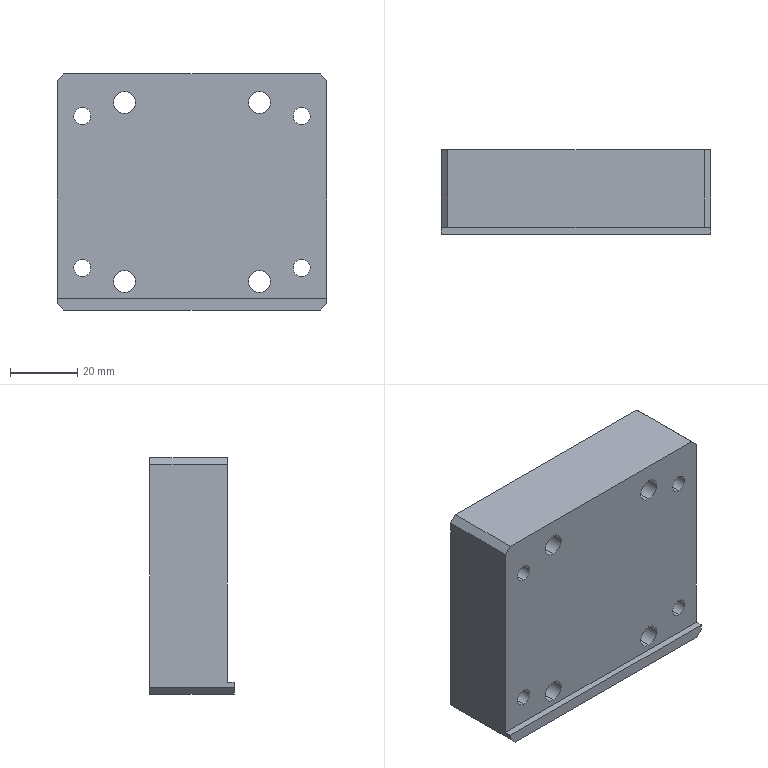Part | SolidWorks | features HoleWzd 3, Chamfer 1, Cut 1, Extrusion 1 | 1 solid | 40 faces | box 80 x 25 x 70 mm | volume 122511 mm3 | cylinder 24 | plane 16 | commonest cylinder face diameters 5 x8 6.6 x8 11 x8
STEP:
#1=CARTESIAN_POINT('',(20.,5.5,-32.));
#2=VERTEX_POINT('',#1);
#3=CARTESIAN_POINT('',(20.,5.5,-21.));
#4=VERTEX_POINT('',#3);
#5=CARTESIAN_POINT('',(20.,5.5,-26.5));
#6=DIRECTION('',(0.,1.,0.));
#7=DIRECTION('',(0.,0.,1.));
#8=AXIS2_PLACEMENT_3D('',#5,#6,#7);
#9=CIRCLE('',#8,5.5);
#10=EDGE_CURVE('',#2,#4,#9,.T.);
#11=ORIENTED_EDGE('',*,*,#10,.F.);
#12=CARTESIAN_POINT('',(20.,12.5,-32.));
#13=VERTEX_POINT('',#12);
#14=CARTESIAN_POINT('',(20.,12.5,-32.));
#15=DIRECTION('',(0.,1.,0.));
#16=VECTOR('',#15,1000.);
#17=LINE('',#14,#16);
#18=EDGE_CURVE('',#2,#13,#17,.T.);
#19=ORIENTED_EDGE('',*,*,#18,.T.);
#20=CARTESIAN_POINT('',(20.,12.5,-21.));
#21=VERTEX_POINT('',#20);
#22=CARTESIAN_POINT('',(20.,12.5,-26.5));
#23=DIRECTION('',(0.,1.,0.));
#24=DIRECTION('',(0.,0.,1.));
#25=AXIS2_PLACEMENT_3D('',#22,#23,#24);
#26=CIRCLE('',#25,5.5);
#27=EDGE_CURVE('',#13,#21,#26,.T.);
#28=ORIENTED_EDGE('',*,*,#27,.T.);
#29=CARTESIAN_POINT('',(20.,12.5,-21.));
#30=DIRECTION('',(0.,1.,0.));
#31=VECTOR('',#30,1000.);
#32=LINE('',#29,#31);
#33=EDGE_CURVE('',#4,#21,#32,.T.);
#34=ORIENTED_EDGE('',*,*,#33,.F.);
#35=EDGE_LOOP('',(#11,#19,#28,#34));
#36=FACE_OUTER_BOUND('',#35,.T.);
#37=CARTESIAN_POINT('',(20.,12.5,-26.5));
#38=DIRECTION('',(0.,1.,0.));
#39=DIRECTION('',(0.,0.,1.));
#40=AXIS2_PLACEMENT_3D('',#37,#38,#39);
#41=CYLINDRICAL_SURFACE('',#40,5.5);
#42=ADVANCED_FACE('',(#36),#41,.F.);
#43=CARTESIAN_POINT('',(20.,-10.5,-29.8));
#44=VERTEX_POINT('',#43);
#45=CARTESIAN_POINT('',(20.,-10.5,-23.2));
#46=VERTEX_POINT('',#45);
#47=CARTESIAN_POINT('',(20.,-10.5,-26.5));
#48=DIRECTION('',(0.,1.,0.));
#49=DIRECTION('',(0.,0.,1.));
#50=AXIS2_PLACEMENT_3D('',#47,#48,#49);
#51=CIRCLE('',#50,3.3);
#52=EDGE_CURVE('',#44,#46,#51,.T.);
#53=ORIENTED_EDGE('',*,*,#52,.F.);
#54=CARTESIAN_POINT('',(20.,5.5,-29.8));
#55=VERTEX_POINT('',#54);
#56=CARTESIAN_POINT('',(20.,12.5,-29.8));
#57=DIRECTION('',(0.,1.,0.));
#58=VECTOR('',#57,1000.);
#59=LINE('',#56,#58);
#60=EDGE_CURVE('',#44,#55,#59,.T.);
#61=ORIENTED_EDGE('',*,*,#60,.T.);
#62=CARTESIAN_POINT('',(20.,5.5,-23.2));
#63=VERTEX_POINT('',#62);
#64=CARTESIAN_POINT('',(20.,5.5,-26.5));
#65=DIRECTION('',(0.,1.,0.));
#66=DIRECTION('',(0.,0.,1.));
#67=AXIS2_PLACEMENT_3D('',#64,#65,#66);
#68=CIRCLE('',#67,3.3);
#69=EDGE_CURVE('',#55,#63,#68,.T.);
#70=ORIENTED_EDGE('',*,*,#69,.T.);
#71=CARTESIAN_POINT('',(20.,12.5,-23.2));
#72=DIRECTION('',(0.,1.,0.));
#73=VECTOR('',#72,1000.);
#74=LINE('',#71,#73);
#75=EDGE_CURVE('',#46,#63,#74,.T.);
#76=ORIENTED_EDGE('',*,*,#75,.F.);
#77=EDGE_LOOP('',(#53,#61,#70,#76));
#78=FACE_OUTER_BOUND('',#77,.T.);
#79=CARTESIAN_POINT('',(20.,12.5,-26.5));
#80=DIRECTION('',(0.,1.,0.));
#81=DIRECTION('',(0.,0.,1.));
#82=AXIS2_PLACEMENT_3D('',#79,#80,#81);
#83=CYLINDRICAL_SURFACE('',#82,3.3);
#84=ADVANCED_FACE('',(#78),#83,.F.);
#85=CARTESIAN_POINT('',(20.,5.5,21.));
#86=VERTEX_POINT('',#85);
#87=CARTESIAN_POINT('',(20.,5.5,32.));
#88=VERTEX_POINT('',#87);
#89=CARTESIAN_POINT('',(20.,5.5,26.5));
#90=DIRECTION('',(0.,1.,0.));
#91=DIRECTION('',(0.,0.,1.));
#92=AXIS2_PLACEMENT_3D('',#89,#90,#91);
#93=CIRCLE('',#92,5.5);
#94=EDGE_CURVE('',#86,#88,#93,.T.);
#95=ORIENTED_EDGE('',*,*,#94,.F.);
#96=CARTESIAN_POINT('',(20.,12.5,21.));
#97=VERTEX_POINT('',#96);
#98=CARTESIAN_POINT('',(20.,12.5,21.));
#99=DIRECTION('',(0.,1.,0.));
#100=VECTOR('',#99,1000.);
#101=LINE('',#98,#100);
#102=EDGE_CURVE('',#86,#97,#101,.T.);
#103=ORIENTED_EDGE('',*,*,#102,.T.);
#104=CARTESIAN_POINT('',(20.,12.5,32.));
#105=VERTEX_POINT('',#104);
#106=CARTESIAN_POINT('',(20.,12.5,26.5));
#107=DIRECTION('',(0.,1.,0.));
#108=DIRECTION('',(0.,0.,1.));
#109=AXIS2_PLACEMENT_3D('',#106,#107,#108);
#110=CIRCLE('',#109,5.5);
#111=EDGE_CURVE('',#97,#105,#110,.T.);
#112=ORIENTED_EDGE('',*,*,#111,.T.);
#113=CARTESIAN_POINT('',(20.,12.5,32.));
#114=DIRECTION('',(0.,1.,0.));
#115=VECTOR('',#114,1000.);
#116=LINE('',#113,#115);
#117=EDGE_CURVE('',#88,#105,#116,.T.);
#118=ORIENTED_EDGE('',*,*,#117,.F.);
#119=EDGE_LOOP('',(#95,#103,#112,#118));
#120=FACE_OUTER_BOUND('',#119,.T.);
#121=CARTESIAN_POINT('',(20.,12.5,26.5));
#122=DIRECTION('',(0.,1.,0.));
#123=DIRECTION('',(0.,0.,1.));
#124=AXIS2_PLACEMENT_3D('',#121,#122,#123);
#125=CYLINDRICAL_SURFACE('',#124,5.5);
#126=ADVANCED_FACE('',(#120),#125,.F.);
#127=CARTESIAN_POINT('',(20.,-10.5,23.2));
#128=VERTEX_POINT('',#127);
#129=CARTESIAN_POINT('',(20.,-10.5,29.8));
#130=VERTEX_POINT('',#129);
#131=CARTESIAN_POINT('',(20.,-10.5,26.5));
#132=DIRECTION('',(0.,1.,0.));
#133=DIRECTION('',(0.,0.,1.));
#134=AXIS2_PLACEMENT_3D('',#131,#132,#133);
#135=CIRCLE('',#134,3.3);
#136=EDGE_CURVE('',#128,#130,#135,.T.);
#137=ORIENTED_EDGE('',*,*,#136,.F.);
#138=CARTESIAN_POINT('',(20.,5.5,23.2));
#139=VERTEX_POINT('',#138);
#140=CARTESIAN_POINT('',(20.,12.5,23.2));
#141=DIRECTION('',(0.,1.,0.));
#142=VECTOR('',#141,1000.);
#143=LINE('',#140,#142);
#144=EDGE_CURVE('',#128,#139,#143,.T.);
#145=ORIENTED_EDGE('',*,*,#144,.T.);
#146=CARTESIAN_POINT('',(20.,5.5,29.8));
#147=VERTEX_POINT('',#146);
#148=CARTESIAN_POINT('',(20.,5.5,26.5));
#149=DIRECTION('',(0.,1.,0.));
#150=DIRECTION('',(0.,0.,1.));
#151=AXIS2_PLACEMENT_3D('',#148,#149,#150);
#152=CIRCLE('',#151,3.3);
#153=EDGE_CURVE('',#139,#147,#152,.T.);
#154=ORIENTED_EDGE('',*,*,#153,.T.);
#155=CARTESIAN_POINT('',(20.,12.5,29.8));
#156=DIRECTION('',(0.,1.,0.));
#157=VECTOR('',#156,1000.);
#158=LINE('',#155,#157);
#159=EDGE_CURVE('',#130,#147,#158,.T.);
#160=ORIENTED_EDGE('',*,*,#159,.F.);
#161=EDGE_LOOP('',(#137,#145,#154,#160));
#162=FACE_OUTER_BOUND('',#161,.T.);
#163=CARTESIAN_POINT('',(20.,12.5,26.5));
#164=DIRECTION('',(0.,1.,0.));
#165=DIRECTION('',(0.,0.,1.));
#166=AXIS2_PLACEMENT_3D('',#163,#164,#165);
#167=CYLINDRICAL_SURFACE('',#166,3.3);
#168=ADVANCED_FACE('',(#162),#167,.F.);
#169=CARTESIAN_POINT('',(-20.,5.5,21.));
#170=VERTEX_POINT('',#169);
#171=CARTESIAN_POINT('',(-20.,5.5,32.));
#172=VERTEX_POINT('',#171);
#173=CARTESIAN_POINT('',(-20.,5.5,26.5));
#174=DIRECTION('',(0.,1.,0.));
#175=DIRECTION('',(0.,0.,1.));
#176=AXIS2_PLACEMENT_3D('',#173,#174,#175);
#177=CIRCLE('',#176,5.5);
#178=EDGE_CURVE('',#170,#172,#177,.T.);
#179=ORIENTED_EDGE('',*,*,#178,.F.);
#180=CARTESIAN_POINT('',(-20.,12.5,21.));
#181=VERTEX_POINT('',#180);
#182=CARTESIAN_POINT('',(-20.,12.5,21.));
#183=DIRECTION('',(0.,1.,0.));
#184=VECTOR('',#183,1000.);
#185=LINE('',#182,#184);
#186=EDGE_CURVE('',#170,#181,#185,.T.);
#187=ORIENTED_EDGE('',*,*,#186,.T.);
#188=CARTESIAN_POINT('',(-20.,12.5,32.));
#189=VERTEX_POINT('',#188);
#190=CARTESIAN_POINT('',(-20.,12.5,26.5));
#191=DIRECTION('',(0.,1.,0.));
#192=DIRECTION('',(0.,0.,1.));
#193=AXIS2_PLACEMENT_3D('',#190,#191,#192);
#194=CIRCLE('',#193,5.5);
#195=EDGE_CURVE('',#181,#189,#194,.T.);
#196=ORIENTED_EDGE('',*,*,#195,.T.);
#197=CARTESIAN_POINT('',(-20.,12.5,32.));
#198=DIRECTION('',(0.,1.,0.));
#199=VECTOR('',#198,1000.);
#200=LINE('',#197,#199);
#201=EDGE_CURVE('',#172,#189,#200,.T.);
#202=ORIENTED_EDGE('',*,*,#201,.F.);
#203=EDGE_LOOP('',(#179,#187,#196,#202));
#204=FACE_OUTER_BOUND('',#203,.T.);
#205=CARTESIAN_POINT('',(-20.,12.5,26.5));
#206=DIRECTION('',(0.,1.,0.));
#207=DIRECTION('',(0.,0.,1.));
#208=AXIS2_PLACEMENT_3D('',#205,#206,#207);
#209=CYLINDRICAL_SURFACE('',#208,5.5);
#210=ADVANCED_FACE('',(#204),#209,.F.);
#211=CARTESIAN_POINT('',(-20.,-10.5,23.2));
#212=VERTEX_POINT('',#211);
#213=CARTESIAN_POINT('',(-20.,-10.5,29.8));
#214=VERTEX_POINT('',#213);
#215=CARTESIAN_POINT('',(-20.,-10.5,26.5));
#216=DIRECTION('',(0.,1.,0.));
#217=DIRECTION('',(0.,0.,1.));
#218=AXIS2_PLACEMENT_3D('',#215,#216,#217);
#219=CIRCLE('',#218,3.3);
#220=EDGE_CURVE('',#212,#214,#219,.T.);
#221=ORIENTED_EDGE('',*,*,#220,.F.);
#222=CARTESIAN_POINT('',(-20.,5.5,23.2));
#223=VERTEX_POINT('',#222);
#224=CARTESIAN_POINT('',(-20.,12.5,23.2));
#225=DIRECTION('',(0.,1.,0.));
#226=VECTOR('',#225,1000.);
#227=LINE('',#224,#226);
#228=EDGE_CURVE('',#212,#223,#227,.T.);
#229=ORIENTED_EDGE('',*,*,#228,.T.);
#230=CARTESIAN_POINT('',(-20.,5.5,29.8));
#231=VERTEX_POINT('',#230);
#232=CARTESIAN_POINT('',(-20.,5.5,26.5));
#233=DIRECTION('',(0.,1.,0.));
#234=DIRECTION('',(0.,0.,1.));
#235=AXIS2_PLACEMENT_3D('',#232,#233,#234);
#236=CIRCLE('',#235,3.3);
#237=EDGE_CURVE('',#223,#231,#236,.T.);
#238=ORIENTED_EDGE('',*,*,#237,.T.);
#239=CARTESIAN_POINT('',(-20.,12.5,29.8));
#240=DIRECTION('',(0.,1.,0.));
#241=VECTOR('',#240,1000.);
#242=LINE('',#239,#241);
#243=EDGE_CURVE('',#214,#231,#242,.T.);
#244=ORIENTED_EDGE('',*,*,#243,.F.);
#245=EDGE_LOOP('',(#221,#229,#238,#244));
#246=FACE_OUTER_BOUND('',#245,.T.);
#247=CARTESIAN_POINT('',(-20.,12.5,26.5));
#248=DIRECTION('',(0.,1.,0.));
#249=DIRECTION('',(0.,0.,1.));
#250=AXIS2_PLACEMENT_3D('',#247,#248,#249);
#251=CYLINDRICAL_SURFACE('',#250,3.3);
#252=ADVANCED_FACE('',(#246),#251,.F.);
#253=CARTESIAN_POINT('',(-20.,5.5,-32.));
#254=VERTEX_POINT('',#253);
#255=CARTESIAN_POINT('',(-20.,5.5,-21.));
#256=VERTEX_POINT('',#255);
#257=CARTESIAN_POINT('',(-20.,5.5,-26.5));
#258=DIRECTION('',(0.,1.,0.));
#259=DIRECTION('',(0.,0.,1.));
#260=AXIS2_PLACEMENT_3D('',#257,#258,#259);
#261=CIRCLE('',#260,5.5);
#262=EDGE_CURVE('',#254,#256,#261,.T.);
#263=ORIENTED_EDGE('',*,*,#262,.F.);
#264=CARTESIAN_POINT('',(-20.,12.5,-32.));
#265=VERTEX_POINT('',#264);
#266=CARTESIAN_POINT('',(-20.,12.5,-32.));
#267=DIRECTION('',(0.,1.,0.));
#268=VECTOR('',#267,1000.);
#269=LINE('',#266,#268);
#270=EDGE_CURVE('',#254,#265,#269,.T.);
#271=ORIENTED_EDGE('',*,*,#270,.T.);
#272=CARTESIAN_POINT('',(-20.,12.5,-21.));
#273=VERTEX_POINT('',#272);
#274=CARTESIAN_POINT('',(-20.,12.5,-26.5));
#275=DIRECTION('',(0.,1.,0.));
#276=DIRECTION('',(0.,0.,1.));
#277=AXIS2_PLACEMENT_3D('',#274,#275,#276);
#278=CIRCLE('',#277,5.5);
#279=EDGE_CURVE('',#265,#273,#278,.T.);
#280=ORIENTED_EDGE('',*,*,#279,.T.);
#281=CARTESIAN_POINT('',(-20.,12.5,-21.));
#282=DIRECTION('',(0.,1.,0.));
#283=VECTOR('',#282,1000.);
#284=LINE('',#281,#283);
#285=EDGE_CURVE('',#256,#273,#284,.T.);
#286=ORIENTED_EDGE('',*,*,#285,.F.);
#287=EDGE_LOOP('',(#263,#271,#280,#286));
#288=FACE_OUTER_BOUND('',#287,.T.);
#289=CARTESIAN_POINT('',(-20.,12.5,-26.5));
#290=DIRECTION('',(0.,1.,0.));
#291=DIRECTION('',(0.,0.,1.));
#292=AXIS2_PLACEMENT_3D('',#289,#290,#291);
#293=CYLINDRICAL_SURFACE('',#292,5.5);
#294=ADVANCED_FACE('',(#288),#293,.F.);
#295=CARTESIAN_POINT('',(-20.,-10.5,-29.8));
#296=VERTEX_POINT('',#295);
#297=CARTESIAN_POINT('',(-20.,-10.5,-23.2));
#298=VERTEX_POINT('',#297);
#299=CARTESIAN_POINT('',(-20.,-10.5,-26.5));
#300=DIRECTION('',(0.,1.,0.));
#301=DIRECTION('',(0.,0.,1.));
#302=AXIS2_PLACEMENT_3D('',#299,#300,#301);
#303=CIRCLE('',#302,3.3);
#304=EDGE_CURVE('',#296,#298,#303,.T.);
#305=ORIENTED_EDGE('',*,*,#304,.F.);
#306=CARTESIAN_POINT('',(-20.,5.5,-29.8));
#307=VERTEX_POINT('',#306);
#308=CARTESIAN_POINT('',(-20.,12.5,-29.8));
#309=DIRECTION('',(0.,1.,0.));
#310=VECTOR('',#309,1000.);
#311=LINE('',#308,#310);
#312=EDGE_CURVE('',#296,#307,#311,.T.);
#313=ORIENTED_EDGE('',*,*,#312,.T.);
#314=CARTESIAN_POINT('',(-20.,5.5,-23.2));
#315=VERTEX_POINT('',#314);
#316=CARTESIAN_POINT('',(-20.,5.5,-26.5));
#317=DIRECTION('',(0.,1.,0.));
#318=DIRECTION('',(0.,0.,1.));
#319=AXIS2_PLACEMENT_3D('',#316,#317,#318);
#320=CIRCLE('',#319,3.3);
#321=EDGE_CURVE('',#307,#315,#320,.T.);
#322=ORIENTED_EDGE('',*,*,#321,.T.);
#323=CARTESIAN_POINT('',(-20.,12.5,-23.2));
#324=DIRECTION('',(0.,1.,0.));
#325=VECTOR('',#324,1000.);
#326=LINE('',#323,#325);
#327=EDGE_CURVE('',#298,#315,#326,.T.);
#328=ORIENTED_EDGE('',*,*,#327,.F.);
#329=EDGE_LOOP('',(#305,#313,#322,#328));
#330=FACE_OUTER_BOUND('',#329,.T.);
#331=CARTESIAN_POINT('',(-20.,12.5,-26.5));
#332=DIRECTION('',(0.,1.,0.));
#333=DIRECTION('',(0.,0.,1.));
#334=AXIS2_PLACEMENT_3D('',#331,#332,#333);
#335=CYLINDRICAL_SURFACE('',#334,3.3);
#336=ADVANCED_FACE('',(#330),#335,.F.);
#337=CARTESIAN_POINT('',(-32.5,12.5,-20.));
#338=VERTEX_POINT('',#337);
#339=CARTESIAN_POINT('',(-32.5,12.5,-25.));
#340=VERTEX_POINT('',#339);
#341=CARTESIAN_POINT('',(-32.5,12.5,-22.5));
#342=DIRECTION('',(0.,-1.,0.));
#343=DIRECTION('',(0.,0.,-1.));
#344=AXIS2_PLACEMENT_3D('',#341,#342,#343);
#345=CIRCLE('',#344,2.5);
#346=EDGE_CURVE('',#338,#340,#345,.T.);
#347=ORIENTED_EDGE('',*,*,#346,.F.);
#348=CARTESIAN_POINT('',(-32.5,-10.5,-20.));
#349=VERTEX_POINT('',#348);
#350=CARTESIAN_POINT('',(-32.5,-10.5,-20.));
#351=DIRECTION('',(0.,-1.,0.));
#352=VECTOR('',#351,1000.);
#353=LINE('',#350,#352);
#354=EDGE_CURVE('',#338,#349,#353,.T.);
#355=ORIENTED_EDGE('',*,*,#354,.T.);
#356=CARTESIAN_POINT('',(-32.5,-10.5,-25.));
#357=VERTEX_POINT('',#356);
#358=CARTESIAN_POINT('',(-32.5,-10.5,-22.5));
#359=DIRECTION('',(0.,-1.,0.));
#360=DIRECTION('',(0.,0.,-1.));
#361=AXIS2_PLACEMENT_3D('',#358,#359,#360);
#362=CIRCLE('',#361,2.5);
#363=EDGE_CURVE('',#349,#357,#362,.T.);
#364=ORIENTED_EDGE('',*,*,#363,.T.);
#365=CARTESIAN_POINT('',(-32.5,-10.5,-25.));
#366=DIRECTION('',(0.,-1.,0.));
#367=VECTOR('',#366,1000.);
#368=LINE('',#365,#367);
#369=EDGE_CURVE('',#340,#357,#368,.T.);
#370=ORIENTED_EDGE('',*,*,#369,.F.);
#371=EDGE_LOOP('',(#347,#355,#364,#370));
#372=FACE_OUTER_BOUND('',#371,.T.);
#373=CARTESIAN_POINT('',(-32.5,-10.5,-22.5));
#374=DIRECTION('',(0.,-1.,0.));
#375=DIRECTION('',(0.,0.,-1.));
#376=AXIS2_PLACEMENT_3D('',#373,#374,#375);
#377=CYLINDRICAL_SURFACE('',#376,2.5);
#378=ADVANCED_FACE('',(#372),#377,.F.);
#379=CARTESIAN_POINT('',(-32.5,12.5,25.));
#380=VERTEX_POINT('',#379);
#381=CARTESIAN_POINT('',(-32.5,12.5,20.));
#382=VERTEX_POINT('',#381);
#383=CARTESIAN_POINT('',(-32.5,12.5,22.5));
#384=DIRECTION('',(0.,-1.,0.));
#385=DIRECTION('',(0.,0.,-1.));
#386=AXIS2_PLACEMENT_3D('',#383,#384,#385);
#387=CIRCLE('',#386,2.5);
#388=EDGE_CURVE('',#380,#382,#387,.T.);
#389=ORIENTED_EDGE('',*,*,#388,.F.);
#390=CARTESIAN_POINT('',(-32.5,-10.5,25.));
#391=VERTEX_POINT('',#390);
#392=CARTESIAN_POINT('',(-32.5,-10.5,25.));
#393=DIRECTION('',(0.,-1.,0.));
#394=VECTOR('',#393,1000.);
#395=LINE('',#392,#394);
#396=EDGE_CURVE('',#380,#391,#395,.T.);
#397=ORIENTED_EDGE('',*,*,#396,.T.);
#398=CARTESIAN_POINT('',(-32.5,-10.5,20.));
#399=VERTEX_POINT('',#398);
#400=CARTESIAN_POINT('',(-32.5,-10.5,22.5));
#401=DIRECTION('',(0.,-1.,0.));
#402=DIRECTION('',(0.,0.,-1.));
#403=AXIS2_PLACEMENT_3D('',#400,#401,#402);
#404=CIRCLE('',#403,2.5);
#405=EDGE_CURVE('',#391,#399,#404,.T.);
#406=ORIENTED_EDGE('',*,*,#405,.T.);
#407=CARTESIAN_POINT('',(-32.5,-10.5,20.));
#408=DIRECTION('',(0.,-1.,0.));
#409=VECTOR('',#408,1000.);
#410=LINE('',#407,#409);
#411=EDGE_CURVE('',#382,#399,#410,.T.);
#412=ORIENTED_EDGE('',*,*,#411,.F.);
#413=EDGE_LOOP('',(#389,#397,#406,#412));
#414=FACE_OUTER_BOUND('',#413,.T.);
#415=CARTESIAN_POINT('',(-32.5,-10.5,22.5));
#416=DIRECTION('',(0.,-1.,0.));
#417=DIRECTION('',(0.,0.,-1.));
#418=AXIS2_PLACEMENT_3D('',#415,#416,#417);
#419=CYLINDRICAL_SURFACE('',#418,2.5);
#420=ADVANCED_FACE('',(#414),#419,.F.);
#421=CARTESIAN_POINT('',(32.5,12.5,-20.));
#422=VERTEX_POINT('',#421);
#423=CARTESIAN_POINT('',(32.5,12.5,-25.));
#424=VERTEX_POINT('',#423);
#425=CARTESIAN_POINT('',(32.5,12.5,-22.5));
#426=DIRECTION('',(0.,-1.,0.));
#427=DIRECTION('',(0.,0.,-1.));
#428=AXIS2_PLACEMENT_3D('',#425,#426,#427);
#429=CIRCLE('',#428,2.5);
#430=EDGE_CURVE('',#422,#424,#429,.T.);
#431=ORIENTED_EDGE('',*,*,#430,.F.);
#432=CARTESIAN_POINT('',(32.5,-10.5,-20.));
#433=VERTEX_POINT('',#432);
#434=CARTESIAN_POINT('',(32.5,-10.5,-20.));
#435=DIRECTION('',(0.,-1.,0.));
#436=VECTOR('',#435,1000.);
#437=LINE('',#434,#436);
#438=EDGE_CURVE('',#422,#433,#437,.T.);
#439=ORIENTED_EDGE('',*,*,#438,.T.);
#440=CARTESIAN_POINT('',(32.5,-10.5,-25.));
#441=VERTEX_POINT('',#440);
#442=CARTESIAN_POINT('',(32.5,-10.5,-22.5));
#443=DIRECTION('',(0.,-1.,0.));
#444=DIRECTION('',(0.,0.,-1.));
#445=AXIS2_PLACEMENT_3D('',#442,#443,#444);
#446=CIRCLE('',#445,2.5);
#447=EDGE_CURVE('',#433,#441,#446,.T.);
#448=ORIENTED_EDGE('',*,*,#447,.T.);
#449=CARTESIAN_POINT('',(32.5,-10.5,-25.));
#450=DIRECTION('',(0.,-1.,0.));
#451=VECTOR('',#450,1000.);
#452=LINE('',#449,#451);
#453=EDGE_CURVE('',#424,#441,#452,.T.);
#454=ORIENTED_EDGE('',*,*,#453,.F.);
#455=EDGE_LOOP('',(#431,#439,#448,#454));
#456=FACE_OUTER_BOUND('',#455,.T.);
#457=CARTESIAN_POINT('',(32.5,-10.5,-22.5));
#458=DIRECTION('',(0.,-1.,0.));
#459=DIRECTION('',(0.,0.,-1.));
#460=AXIS2_PLACEMENT_3D('',#457,#458,#459);
#461=CYLINDRICAL_SURFACE('',#460,2.5);
#462=ADVANCED_FACE('',(#456),#461,.F.);
#463=CARTESIAN_POINT('',(32.5,12.5,25.));
#464=VERTEX_POINT('',#463);
#465=CARTESIAN_POINT('',(32.5,12.5,20.));
#466=VERTEX_POINT('',#465);
#467=CARTESIAN_POINT('',(32.5,12.5,22.5));
#468=DIRECTION('',(0.,-1.,0.));
#469=DIRECTION('',(0.,0.,-1.));
#470=AXIS2_PLACEMENT_3D('',#467,#468,#469);
#471=CIRCLE('',#470,2.5);
#472=EDGE_CURVE('',#464,#466,#471,.T.);
#473=ORIENTED_EDGE('',*,*,#472,.F.);
#474=CARTESIAN_POINT('',(32.5,-10.5,25.));
#475=VERTEX_POINT('',#474);
#476=CARTESIAN_POINT('',(32.5,-10.5,25.));
#477=DIRECTION('',(0.,-1.,0.));
#478=VECTOR('',#477,1000.);
#479=LINE('',#476,#478);
#480=EDGE_CURVE('',#464,#475,#479,.T.);
#481=ORIENTED_EDGE('',*,*,#480,.T.);
#482=CARTESIAN_POINT('',(32.5,-10.5,20.));
#483=VERTEX_POINT('',#482);
#484=CARTESIAN_POINT('',(32.5,-10.5,22.5));
#485=DIRECTION('',(0.,-1.,0.));
#486=DIRECTION('',(0.,0.,-1.));
#487=AXIS2_PLACEMENT_3D('',#484,#485,#486);
#488=CIRCLE('',#487,2.5);
#489=EDGE_CURVE('',#475,#483,#488,.T.);
#490=ORIENTED_EDGE('',*,*,#489,.T.);
#491=CARTESIAN_POINT('',(32.5,-10.5,20.));
#492=DIRECTION('',(0.,-1.,0.));
#493=VECTOR('',#492,1000.);
#494=LINE('',#491,#493);
#495=EDGE_CURVE('',#466,#483,#494,.T.);
#496=ORIENTED_EDGE('',*,*,#495,.F.);
#497=EDGE_LOOP('',(#473,#481,#490,#496));
#498=FACE_OUTER_BOUND('',#497,.T.);
#499=CARTESIAN_POINT('',(32.5,-10.5,22.5));
#500=DIRECTION('',(0.,-1.,0.));
#501=DIRECTION('',(0.,0.,-1.));
#502=AXIS2_PLACEMENT_3D('',#499,#500,#501);
#503=CYLINDRICAL_SURFACE('',#502,2.5);
#504=ADVANCED_FACE('',(#498),#503,.F.);
#505=CARTESIAN_POINT('',(-40.,-10.5,33.));
#506=VERTEX_POINT('',#505);
#507=CARTESIAN_POINT('',(-40.,-10.5,-31.5));
#508=VERTEX_POINT('',#507);
#509=CARTESIAN_POINT('',(-40.,-10.5,35.));
#510=DIRECTION('',(0.,0.,-1.));
#511=VECTOR('',#510,1000.);
#512=LINE('',#509,#511);
#513=EDGE_CURVE('',#506,#508,#512,.T.);
#514=ORIENTED_EDGE('',*,*,#513,.F.);
#515=CARTESIAN_POINT('',(-40.,12.5,33.));
#516=VERTEX_POINT('',#515);
#517=CARTESIAN_POINT('',(-40.,12.5,33.));
#518=DIRECTION('',(0.,1.,0.));
#519=VECTOR('',#518,1000.);
#520=LINE('',#517,#519);
#521=EDGE_CURVE('',#506,#516,#520,.T.);
#522=ORIENTED_EDGE('',*,*,#521,.T.);
#523=CARTESIAN_POINT('',(-40.,12.5,-33.));
#524=VERTEX_POINT('',#523);
#525=CARTESIAN_POINT('',(-40.,12.5,35.));
#526=DIRECTION('',(0.,0.,1.));
#527=VECTOR('',#526,1000.);
#528=LINE('',#525,#527);
#529=EDGE_CURVE('',#524,#516,#528,.T.);
#530=ORIENTED_EDGE('',*,*,#529,.F.);
#531=CARTESIAN_POINT('',(-40.,-12.5,-33.));
#532=VERTEX_POINT('',#531);
#533=CARTESIAN_POINT('',(-40.,12.5,-33.));
#534=DIRECTION('',(0.,-1.,0.));
#535=VECTOR('',#534,1000.);
#536=LINE('',#533,#535);
#537=EDGE_CURVE('',#524,#532,#536,.T.);
#538=ORIENTED_EDGE('',*,*,#537,.T.);
#539=CARTESIAN_POINT('',(-40.,-12.5,-31.5));
#540=VERTEX_POINT('',#539);
#541=CARTESIAN_POINT('',(-40.,-12.5,35.));
#542=DIRECTION('',(0.,0.,1.));
#543=VECTOR('',#542,1000.);
#544=LINE('',#541,#543);
#545=EDGE_CURVE('',#532,#540,#544,.T.);
#546=ORIENTED_EDGE('',*,*,#545,.T.);
#547=CARTESIAN_POINT('',(-40.,-10.5,-31.5));
#548=DIRECTION('',(0.,-1.,0.));
#549=VECTOR('',#548,1000.);
#550=LINE('',#547,#549);
#551=EDGE_CURVE('',#508,#540,#550,.T.);
#552=ORIENTED_EDGE('',*,*,#551,.F.);
#553=EDGE_LOOP('',(#514,#522,#530,#538,#546,#552));
#554=FACE_OUTER_BOUND('',#553,.T.);
#555=CARTESIAN_POINT('',(-40.,12.5,35.));
#556=DIRECTION('',(1.,0.,0.));
#557=DIRECTION('',(0.,0.,-1.));
#558=AXIS2_PLACEMENT_3D('',#555,#556,#557);
#559=PLANE('',#558);
#560=ADVANCED_FACE('',(#554),#559,.F.);
#561=CARTESIAN_POINT('',(-38.,12.5,35.));
#562=VERTEX_POINT('',#561);
#563=CARTESIAN_POINT('',(38.,12.5,35.));
#564=VERTEX_POINT('',#563);
#565=CARTESIAN_POINT('',(40.,12.5,35.));
#566=DIRECTION('',(1.,0.,0.));
#567=VECTOR('',#566,1000.);
#568=LINE('',#565,#567);
#569=EDGE_CURVE('',#562,#564,#568,.T.);
#570=ORIENTED_EDGE('',*,*,#569,.F.);
#571=CARTESIAN_POINT('',(-38.,-10.5,35.));
#572=VERTEX_POINT('',#571);
#573=CARTESIAN_POINT('',(-38.,12.5,35.));
#574=DIRECTION('',(0.,-1.,0.));
#575=VECTOR('',#574,1000.);
#576=LINE('',#573,#575);
#577=EDGE_CURVE('',#562,#572,#576,.T.);
#578=ORIENTED_EDGE('',*,*,#577,.T.);
#579=CARTESIAN_POINT('',(38.,-10.5,35.));
#580=VERTEX_POINT('',#579);
#581=CARTESIAN_POINT('',(40.,-10.5,35.));
#582=DIRECTION('',(-1.,0.,0.));
#583=VECTOR('',#582,1000.);
#584=LINE('',#581,#583);
#585=EDGE_CURVE('',#580,#572,#584,.T.);
#586=ORIENTED_EDGE('',*,*,#585,.F.);
#587=CARTESIAN_POINT('',(38.,12.5,35.));
#588=DIRECTION('',(0.,1.,0.));
#589=VECTOR('',#588,1000.);
#590=LINE('',#587,#589);
#591=EDGE_CURVE('',#580,#564,#590,.T.);
#592=ORIENTED_EDGE('',*,*,#591,.T.);
#593=EDGE_LOOP('',(#570,#578,#586,#592));
#594=FACE_OUTER_BOUND('',#593,.T.);
#595=CARTESIAN_POINT('',(40.,12.5,35.));
#596=DIRECTION('',(0.,0.,-1.));
#597=DIRECTION('',(-1.,0.,0.));
#598=AXIS2_PLACEMENT_3D('',#595,#596,#597);
#599=PLANE('',#598);
#600=ADVANCED_FACE('',(#594),#599,.F.);
#601=CARTESIAN_POINT('',(40.,12.5,33.));
#602=VERTEX_POINT('',#601);
#603=CARTESIAN_POINT('',(40.,12.5,-33.));
#604=VERTEX_POINT('',#603);
#605=CARTESIAN_POINT('',(40.,12.5,35.));
#606=DIRECTION('',(0.,0.,-1.));
#607=VECTOR('',#606,1000.);
#608=LINE('',#605,#607);
#609=EDGE_CURVE('',#602,#604,#608,.T.);
#610=ORIENTED_EDGE('',*,*,#609,.F.);
#611=CARTESIAN_POINT('',(40.,-10.5,33.));
#612=VERTEX_POINT('',#611);
#613=CARTESIAN_POINT('',(40.,12.5,33.));
#614=DIRECTION('',(0.,-1.,0.));
#615=VECTOR('',#614,1000.);
#616=LINE('',#613,#615);
#617=EDGE_CURVE('',#602,#612,#616,.T.);
#618=ORIENTED_EDGE('',*,*,#617,.T.);
#619=CARTESIAN_POINT('',(40.,-10.5,-31.5));
#620=VERTEX_POINT('',#619);
#621=CARTESIAN_POINT('',(40.,-10.5,35.));
#622=DIRECTION('',(0.,0.,1.));
#623=VECTOR('',#622,1000.);
#624=LINE('',#621,#623);
#625=EDGE_CURVE('',#620,#612,#624,.T.);
#626=ORIENTED_EDGE('',*,*,#625,.F.);
#627=CARTESIAN_POINT('',(40.,-12.5,-31.5));
#628=VERTEX_POINT('',#627);
#629=CARTESIAN_POINT('',(40.,-10.5,-31.5));
#630=DIRECTION('',(0.,-1.,0.));
#631=VECTOR('',#630,1000.);
#632=LINE('',#629,#631);
#633=EDGE_CURVE('',#620,#628,#632,.T.);
#634=ORIENTED_EDGE('',*,*,#633,.T.);
#635=CARTESIAN_POINT('',(40.,-12.5,-33.));
#636=VERTEX_POINT('',#635);
#637=CARTESIAN_POINT('',(40.,-12.5,35.));
#638=DIRECTION('',(0.,0.,-1.));
#639=VECTOR('',#638,1000.);
#640=LINE('',#637,#639);
#641=EDGE_CURVE('',#628,#636,#640,.T.);
#642=ORIENTED_EDGE('',*,*,#641,.T.);
#643=CARTESIAN_POINT('',(40.,12.5,-33.));
#644=DIRECTION('',(0.,1.,0.));
#645=VECTOR('',#644,1000.);
#646=LINE('',#643,#645);
#647=EDGE_CURVE('',#636,#604,#646,.T.);
#648=ORIENTED_EDGE('',*,*,#647,.T.);
#649=EDGE_LOOP('',(#610,#618,#626,#634,#642,#648));
#650=FACE_OUTER_BOUND('',#649,.T.);
#651=CARTESIAN_POINT('',(40.,12.5,35.));
#652=DIRECTION('',(-1.,0.,0.));
#653=DIRECTION('',(0.,0.,1.));
#654=AXIS2_PLACEMENT_3D('',#651,#652,#653);
#655=PLANE('',#654);
#656=ADVANCED_FACE('',(#650),#655,.F.);
#657=CARTESIAN_POINT('',(38.,12.5,-35.));
#658=VERTEX_POINT('',#657);
#659=CARTESIAN_POINT('',(-38.,12.5,-35.));
#660=VERTEX_POINT('',#659);
#661=CARTESIAN_POINT('',(40.,12.5,-35.));
#662=DIRECTION('',(-1.,0.,0.));
#663=VECTOR('',#662,1000.);
#664=LINE('',#661,#663);
#665=EDGE_CURVE('',#658,#660,#664,.T.);
#666=ORIENTED_EDGE('',*,*,#665,.F.);
#667=CARTESIAN_POINT('',(38.,-12.5,-35.));
#668=VERTEX_POINT('',#667);
#669=CARTESIAN_POINT('',(38.,12.5,-35.));
#670=DIRECTION('',(0.,-1.,0.));
#671=VECTOR('',#670,1000.);
#672=LINE('',#669,#671);
#673=EDGE_CURVE('',#658,#668,#672,.T.);
#674=ORIENTED_EDGE('',*,*,#673,.T.);
#675=CARTESIAN_POINT('',(-38.,-12.5,-35.));
#676=VERTEX_POINT('',#675);
#677=CARTESIAN_POINT('',(40.,-12.5,-35.));
#678=DIRECTION('',(-1.,0.,0.));
#679=VECTOR('',#678,1000.);
#680=LINE('',#677,#679);
#681=EDGE_CURVE('',#668,#676,#680,.T.);
#682=ORIENTED_EDGE('',*,*,#681,.T.);
#683=CARTESIAN_POINT('',(-38.,12.5,-35.));
#684=DIRECTION('',(0.,1.,0.));
#685=VECTOR('',#684,1000.);
#686=LINE('',#683,#685);
#687=EDGE_CURVE('',#676,#660,#686,.T.);
#688=ORIENTED_EDGE('',*,*,#687,.T.);
#689=EDGE_LOOP('',(#666,#674,#682,#688));
#690=FACE_OUTER_BOUND('',#689,.T.);
#691=CARTESIAN_POINT('',(40.,12.5,-35.));
#692=DIRECTION('',(0.,0.,1.));
#693=DIRECTION('',(1.,0.,0.));
#694=AXIS2_PLACEMENT_3D('',#691,#692,#693);
#695=PLANE('',#694);
#696=ADVANCED_FACE('',(#690),#695,.F.);
#697=CARTESIAN_POINT('',(20.,12.5,-26.5));
#698=DIRECTION('',(0.,1.,0.));
#699=DIRECTION('',(0.,0.,1.));
#700=AXIS2_PLACEMENT_3D('',#697,#698,#699);
#701=CIRCLE('',#700,5.5);
#702=EDGE_CURVE('',#21,#13,#701,.T.);
#703=ORIENTED_EDGE('',*,*,#702,.F.);
#704=ORIENTED_EDGE('',*,*,#27,.F.);
#705=EDGE_LOOP('',(#703,#704));
#706=FACE_BOUND('',#705,.T.);
#707=CARTESIAN_POINT('',(20.,12.5,26.5));
#708=DIRECTION('',(0.,1.,0.));
#709=DIRECTION('',(0.,0.,1.));
#710=AXIS2_PLACEMENT_3D('',#707,#708,#709);
#711=CIRCLE('',#710,5.5);
#712=EDGE_CURVE('',#105,#97,#711,.T.);
#713=ORIENTED_EDGE('',*,*,#712,.F.);
#714=ORIENTED_EDGE('',*,*,#111,.F.);
#715=EDGE_LOOP('',(#713,#714));
#716=FACE_BOUND('',#715,.T.);
#717=CARTESIAN_POINT('',(-20.,12.5,26.5));
#718=DIRECTION('',(0.,1.,0.));
#719=DIRECTION('',(0.,0.,1.));
#720=AXIS2_PLACEMENT_3D('',#717,#718,#719);
#721=CIRCLE('',#720,5.5);
#722=EDGE_CURVE('',#189,#181,#721,.T.);
#723=ORIENTED_EDGE('',*,*,#722,.F.);
#724=ORIENTED_EDGE('',*,*,#195,.F.);
#725=EDGE_LOOP('',(#723,#724));
#726=FACE_BOUND('',#725,.T.);
#727=CARTESIAN_POINT('',(-20.,12.5,-26.5));
#728=DIRECTION('',(0.,1.,0.));
#729=DIRECTION('',(0.,0.,1.));
#730=AXIS2_PLACEMENT_3D('',#727,#728,#729);
#731=CIRCLE('',#730,5.5);
#732=EDGE_CURVE('',#273,#265,#731,.T.);
#733=ORIENTED_EDGE('',*,*,#732,.F.);
#734=ORIENTED_EDGE('',*,*,#279,.F.);
#735=EDGE_LOOP('',(#733,#734));
#736=FACE_BOUND('',#735,.T.);
#737=CARTESIAN_POINT('',(-32.5,12.5,-22.5));
#738=DIRECTION('',(0.,-1.,0.));
#739=DIRECTION('',(0.,0.,-1.));
#740=AXIS2_PLACEMENT_3D('',#737,#738,#739);
#741=CIRCLE('',#740,2.5);
#742=EDGE_CURVE('',#340,#338,#741,.T.);
#743=ORIENTED_EDGE('',*,*,#742,.T.);
#744=ORIENTED_EDGE('',*,*,#346,.T.);
#745=EDGE_LOOP('',(#743,#744));
#746=FACE_BOUND('',#745,.T.);
#747=CARTESIAN_POINT('',(-32.5,12.5,22.5));
#748=DIRECTION('',(0.,-1.,0.));
#749=DIRECTION('',(0.,0.,-1.));
#750=AXIS2_PLACEMENT_3D('',#747,#748,#749);
#751=CIRCLE('',#750,2.5);
#752=EDGE_CURVE('',#382,#380,#751,.T.);
#753=ORIENTED_EDGE('',*,*,#752,.T.);
#754=ORIENTED_EDGE('',*,*,#388,.T.);
#755=EDGE_LOOP('',(#753,#754));
#756=FACE_BOUND('',#755,.T.);
#757=CARTESIAN_POINT('',(32.5,12.5,-22.5));
#758=DIRECTION('',(0.,-1.,0.));
#759=DIRECTION('',(0.,0.,-1.));
#760=AXIS2_PLACEMENT_3D('',#757,#758,#759);
#761=CIRCLE('',#760,2.5);
#762=EDGE_CURVE('',#424,#422,#761,.T.);
#763=ORIENTED_EDGE('',*,*,#762,.T.);
#764=ORIENTED_EDGE('',*,*,#430,.T.);
#765=EDGE_LOOP('',(#763,#764));
#766=FACE_BOUND('',#765,.T.);
#767=CARTESIAN_POINT('',(32.5,12.5,22.5));
#768=DIRECTION('',(0.,-1.,0.));
#769=DIRECTION('',(0.,0.,-1.));
#770=AXIS2_PLACEMENT_3D('',#767,#768,#769);
#771=CIRCLE('',#770,2.5);
#772=EDGE_CURVE('',#466,#464,#771,.T.);
#773=ORIENTED_EDGE('',*,*,#772,.T.);
#774=ORIENTED_EDGE('',*,*,#472,.T.);
#775=EDGE_LOOP('',(#773,#774));
#776=FACE_BOUND('',#775,.T.);
#777=ORIENTED_EDGE('',*,*,#529,.T.);
#778=CARTESIAN_POINT('',(-36.5,12.5,36.5));
#779=DIRECTION('',(0.7071,0.,0.7071));
#780=VECTOR('',#779,1000.);
#781=LINE('',#778,#780);
#782=EDGE_CURVE('',#516,#562,#781,.T.);
#783=ORIENTED_EDGE('',*,*,#782,.T.);
#784=ORIENTED_EDGE('',*,*,#569,.T.);
#785=CARTESIAN_POINT('',(36.5,12.5,36.5));
#786=DIRECTION('',(0.7071,0.,-0.7071));
#787=VECTOR('',#786,1000.);
#788=LINE('',#785,#787);
#789=EDGE_CURVE('',#564,#602,#788,.T.);
#790=ORIENTED_EDGE('',*,*,#789,.T.);
#791=ORIENTED_EDGE('',*,*,#609,.T.);
#792=CARTESIAN_POINT('',(36.5,12.5,-36.5));
#793=DIRECTION('',(-0.7071,0.,-0.7071));
#794=VECTOR('',#793,1000.);
#795=LINE('',#792,#794);
#796=EDGE_CURVE('',#604,#658,#795,.T.);
#797=ORIENTED_EDGE('',*,*,#796,.T.);
#798=ORIENTED_EDGE('',*,*,#665,.T.);
#799=CARTESIAN_POINT('',(-36.5,12.5,-36.5));
#800=DIRECTION('',(-0.7071,0.,0.7071));
#801=VECTOR('',#800,1000.);
#802=LINE('',#799,#801);
#803=EDGE_CURVE('',#660,#524,#802,.T.);
#804=ORIENTED_EDGE('',*,*,#803,.T.);
#805=EDGE_LOOP('',(#777,#783,#784,#790,#791,#797,#798,#804));
#806=FACE_OUTER_BOUND('',#805,.T.);
#807=CARTESIAN_POINT('',(0.,12.5,0.));
#808=DIRECTION('',(0.,1.,0.));
#809=DIRECTION('',(0.,0.,1.));
#810=AXIS2_PLACEMENT_3D('',#807,#808,#809);
#811=PLANE('',#810);
#812=ADVANCED_FACE('',(#706,#716,#726,#736,#746,#756,#766,#776,#806),#811,.T.);
#813=ORIENTED_EDGE('',*,*,#681,.F.);
#814=CARTESIAN_POINT('',(38.,-12.5,-35.));
#815=DIRECTION('',(0.7071,0.,0.7071));
#816=VECTOR('',#815,1000.);
#817=LINE('',#814,#816);
#818=EDGE_CURVE('',#668,#636,#817,.T.);
#819=ORIENTED_EDGE('',*,*,#818,.T.);
#820=ORIENTED_EDGE('',*,*,#641,.F.);
#821=CARTESIAN_POINT('',(40.,-12.5,-31.5));
#822=DIRECTION('',(1.,0.,0.));
#823=VECTOR('',#822,1000.);
#824=LINE('',#821,#823);
#825=EDGE_CURVE('',#540,#628,#824,.T.);
#826=ORIENTED_EDGE('',*,*,#825,.F.);
#827=ORIENTED_EDGE('',*,*,#545,.F.);
#828=CARTESIAN_POINT('',(-40.,-12.5,-33.));
#829=DIRECTION('',(0.7071,0.,-0.7071));
#830=VECTOR('',#829,1000.);
#831=LINE('',#828,#830);
#832=EDGE_CURVE('',#532,#676,#831,.T.);
#833=ORIENTED_EDGE('',*,*,#832,.T.);
#834=EDGE_LOOP('',(#813,#819,#820,#826,#827,#833));
#835=FACE_OUTER_BOUND('',#834,.T.);
#836=CARTESIAN_POINT('',(0.,-12.5,0.));
#837=DIRECTION('',(0.,1.,0.));
#838=DIRECTION('',(0.,0.,1.));
#839=AXIS2_PLACEMENT_3D('',#836,#837,#838);
#840=PLANE('',#839);
#841=ADVANCED_FACE('',(#835),#840,.F.);
#842=ORIENTED_EDGE('',*,*,#825,.T.);
#843=ORIENTED_EDGE('',*,*,#633,.F.);
#844=CARTESIAN_POINT('',(40.,-10.5,-31.5));
#845=DIRECTION('',(1.,0.,0.));
#846=VECTOR('',#845,1000.);
#847=LINE('',#844,#846);
#848=EDGE_CURVE('',#508,#620,#847,.T.);
#849=ORIENTED_EDGE('',*,*,#848,.F.);
#850=ORIENTED_EDGE('',*,*,#551,.T.);
#851=EDGE_LOOP('',(#842,#843,#849,#850));
#852=FACE_OUTER_BOUND('',#851,.T.);
#853=CARTESIAN_POINT('',(40.,-10.5,-31.5));
#854=DIRECTION('',(0.,0.,-1.));
#855=DIRECTION('',(-1.,0.,0.));
#856=AXIS2_PLACEMENT_3D('',#853,#854,#855);
#857=PLANE('',#856);
#858=ADVANCED_FACE('',(#852),#857,.F.);
#859=CARTESIAN_POINT('',(20.,-10.5,-26.5));
#860=DIRECTION('',(0.,1.,0.));
#861=DIRECTION('',(0.,0.,1.));
#862=AXIS2_PLACEMENT_3D('',#859,#860,#861);
#863=CIRCLE('',#862,3.3);
#864=EDGE_CURVE('',#46,#44,#863,.T.);
#865=ORIENTED_EDGE('',*,*,#864,.T.);
#866=ORIENTED_EDGE('',*,*,#52,.T.);
#867=EDGE_LOOP('',(#865,#866));
#868=FACE_BOUND('',#867,.T.);
#869=CARTESIAN_POINT('',(20.,-10.5,26.5));
#870=DIRECTION('',(0.,1.,0.));
#871=DIRECTION('',(0.,0.,1.));
#872=AXIS2_PLACEMENT_3D('',#869,#870,#871);
#873=CIRCLE('',#872,3.3);
#874=EDGE_CURVE('',#130,#128,#873,.T.);
#875=ORIENTED_EDGE('',*,*,#874,.T.);
#876=ORIENTED_EDGE('',*,*,#136,.T.);
#877=EDGE_LOOP('',(#875,#876));
#878=FACE_BOUND('',#877,.T.);
#879=CARTESIAN_POINT('',(-20.,-10.5,26.5));
#880=DIRECTION('',(0.,1.,0.));
#881=DIRECTION('',(0.,0.,1.));
#882=AXIS2_PLACEMENT_3D('',#879,#880,#881);
#883=CIRCLE('',#882,3.3);
#884=EDGE_CURVE('',#214,#212,#883,.T.);
#885=ORIENTED_EDGE('',*,*,#884,.T.);
#886=ORIENTED_EDGE('',*,*,#220,.T.);
#887=EDGE_LOOP('',(#885,#886));
#888=FACE_BOUND('',#887,.T.);
#889=CARTESIAN_POINT('',(-20.,-10.5,-26.5));
#890=DIRECTION('',(0.,1.,0.));
#891=DIRECTION('',(0.,0.,1.));
#892=AXIS2_PLACEMENT_3D('',#889,#890,#891);
#893=CIRCLE('',#892,3.3);
#894=EDGE_CURVE('',#298,#296,#893,.T.);
#895=ORIENTED_EDGE('',*,*,#894,.T.);
#896=ORIENTED_EDGE('',*,*,#304,.T.);
#897=EDGE_LOOP('',(#895,#896));
#898=FACE_BOUND('',#897,.T.);
#899=CARTESIAN_POINT('',(-32.5,-10.5,-22.5));
#900=DIRECTION('',(0.,-1.,0.));
#901=DIRECTION('',(0.,0.,-1.));
#902=AXIS2_PLACEMENT_3D('',#899,#900,#901);
#903=CIRCLE('',#902,2.5);
#904=EDGE_CURVE('',#357,#349,#903,.T.);
#905=ORIENTED_EDGE('',*,*,#904,.F.);
#906=ORIENTED_EDGE('',*,*,#363,.F.);
#907=EDGE_LOOP('',(#905,#906));
#908=FACE_BOUND('',#907,.T.);
#909=CARTESIAN_POINT('',(-32.5,-10.5,22.5));
#910=DIRECTION('',(0.,-1.,0.));
#911=DIRECTION('',(0.,0.,-1.));
#912=AXIS2_PLACEMENT_3D('',#909,#910,#911);
#913=CIRCLE('',#912,2.5);
#914=EDGE_CURVE('',#399,#391,#913,.T.);
#915=ORIENTED_EDGE('',*,*,#914,.F.);
#916=ORIENTED_EDGE('',*,*,#405,.F.);
#917=EDGE_LOOP('',(#915,#916));
#918=FACE_BOUND('',#917,.T.);
#919=CARTESIAN_POINT('',(32.5,-10.5,-22.5));
#920=DIRECTION('',(0.,-1.,0.));
#921=DIRECTION('',(0.,0.,-1.));
#922=AXIS2_PLACEMENT_3D('',#919,#920,#921);
#923=CIRCLE('',#922,2.5);
#924=EDGE_CURVE('',#441,#433,#923,.T.);
#925=ORIENTED_EDGE('',*,*,#924,.F.);
#926=ORIENTED_EDGE('',*,*,#447,.F.);
#927=EDGE_LOOP('',(#925,#926));
#928=FACE_BOUND('',#927,.T.);
#929=CARTESIAN_POINT('',(32.5,-10.5,22.5));
#930=DIRECTION('',(0.,-1.,0.));
#931=DIRECTION('',(0.,0.,-1.));
#932=AXIS2_PLACEMENT_3D('',#929,#930,#931);
#933=CIRCLE('',#932,2.5);
#934=EDGE_CURVE('',#483,#475,#933,.T.);
#935=ORIENTED_EDGE('',*,*,#934,.F.);
#936=ORIENTED_EDGE('',*,*,#489,.F.);
#937=EDGE_LOOP('',(#935,#936));
#938=FACE_BOUND('',#937,.T.);
#939=ORIENTED_EDGE('',*,*,#585,.T.);
#940=CARTESIAN_POINT('',(-38.,-10.5,35.));
#941=DIRECTION('',(-0.7071,0.,-0.7071));
#942=VECTOR('',#941,1000.);
#943=LINE('',#940,#942);
#944=EDGE_CURVE('',#572,#506,#943,.T.);
#945=ORIENTED_EDGE('',*,*,#944,.T.);
#946=ORIENTED_EDGE('',*,*,#513,.T.);
#947=ORIENTED_EDGE('',*,*,#848,.T.);
#948=ORIENTED_EDGE('',*,*,#625,.T.);
#949=CARTESIAN_POINT('',(40.,-10.5,33.));
#950=DIRECTION('',(-0.7071,0.,0.7071));
#951=VECTOR('',#950,1000.);
#952=LINE('',#949,#951);
#953=EDGE_CURVE('',#612,#580,#952,.T.);
#954=ORIENTED_EDGE('',*,*,#953,.T.);
#955=EDGE_LOOP('',(#939,#945,#946,#947,#948,#954));
#956=FACE_OUTER_BOUND('',#955,.T.);
#957=CARTESIAN_POINT('',(0.,-10.5,0.));
#958=DIRECTION('',(0.,1.,0.));
#959=DIRECTION('',(0.,0.,1.));
#960=AXIS2_PLACEMENT_3D('',#957,#958,#959);
#961=PLANE('',#960);
#962=ADVANCED_FACE('',(#868,#878,#888,#898,#908,#918,#928,#938,#956),#961,.F.);
#963=ORIENTED_EDGE('',*,*,#480,.F.);
#964=ORIENTED_EDGE('',*,*,#772,.F.);
#965=ORIENTED_EDGE('',*,*,#495,.T.);
#966=ORIENTED_EDGE('',*,*,#934,.T.);
#967=EDGE_LOOP('',(#963,#964,#965,#966));
#968=FACE_OUTER_BOUND('',#967,.T.);
#969=CARTESIAN_POINT('',(32.5,-10.5,22.5));
#970=DIRECTION('',(0.,-1.,0.));
#971=DIRECTION('',(0.,0.,-1.));
#972=AXIS2_PLACEMENT_3D('',#969,#970,#971);
#973=CYLINDRICAL_SURFACE('',#972,2.5);
#974=ADVANCED_FACE('',(#968),#973,.F.);
#975=ORIENTED_EDGE('',*,*,#438,.F.);
#976=ORIENTED_EDGE('',*,*,#762,.F.);
#977=ORIENTED_EDGE('',*,*,#453,.T.);
#978=ORIENTED_EDGE('',*,*,#924,.T.);
#979=EDGE_LOOP('',(#975,#976,#977,#978));
#980=FACE_OUTER_BOUND('',#979,.T.);
#981=CARTESIAN_POINT('',(32.5,-10.5,-22.5));
#982=DIRECTION('',(0.,-1.,0.));
#983=DIRECTION('',(0.,0.,-1.));
#984=AXIS2_PLACEMENT_3D('',#981,#982,#983);
#985=CYLINDRICAL_SURFACE('',#984,2.5);
#986=ADVANCED_FACE('',(#980),#985,.F.);
#987=ORIENTED_EDGE('',*,*,#396,.F.);
#988=ORIENTED_EDGE('',*,*,#752,.F.);
#989=ORIENTED_EDGE('',*,*,#411,.T.);
#990=ORIENTED_EDGE('',*,*,#914,.T.);
#991=EDGE_LOOP('',(#987,#988,#989,#990));
#992=FACE_OUTER_BOUND('',#991,.T.);
#993=CARTESIAN_POINT('',(-32.5,-10.5,22.5));
#994=DIRECTION('',(0.,-1.,0.));
#995=DIRECTION('',(0.,0.,-1.));
#996=AXIS2_PLACEMENT_3D('',#993,#994,#995);
#997=CYLINDRICAL_SURFACE('',#996,2.5);
#998=ADVANCED_FACE('',(#992),#997,.F.);
#999=ORIENTED_EDGE('',*,*,#354,.F.);
#1000=ORIENTED_EDGE('',*,*,#742,.F.);
#1001=ORIENTED_EDGE('',*,*,#369,.T.);
#1002=ORIENTED_EDGE('',*,*,#904,.T.);
#1003=EDGE_LOOP('',(#999,#1000,#1001,#1002));
#1004=FACE_OUTER_BOUND('',#1003,.T.);
#1005=CARTESIAN_POINT('',(-32.5,-10.5,-22.5));
#1006=DIRECTION('',(0.,-1.,0.));
#1007=DIRECTION('',(0.,0.,-1.));
#1008=AXIS2_PLACEMENT_3D('',#1005,#1006,#1007);
#1009=CYLINDRICAL_SURFACE('',#1008,2.5);
#1010=ADVANCED_FACE('',(#1004),#1009,.F.);
#1011=ORIENTED_EDGE('',*,*,#782,.F.);
#1012=ORIENTED_EDGE('',*,*,#521,.F.);
#1013=ORIENTED_EDGE('',*,*,#944,.F.);
#1014=ORIENTED_EDGE('',*,*,#577,.F.);
#1015=EDGE_LOOP('',(#1011,#1012,#1013,#1014));
#1016=FACE_OUTER_BOUND('',#1015,.T.);
#1017=CARTESIAN_POINT('',(-38.,12.5,35.));
#1018=DIRECTION('',(0.7071,0.,-0.7071));
#1019=DIRECTION('',(0.,-1.,0.));
#1020=AXIS2_PLACEMENT_3D('',#1017,#1018,#1019);
#1021=PLANE('',#1020);
#1022=ADVANCED_FACE('',(#1016),#1021,.F.);
#1023=ORIENTED_EDGE('',*,*,#789,.F.);
#1024=ORIENTED_EDGE('',*,*,#591,.F.);
#1025=ORIENTED_EDGE('',*,*,#953,.F.);
#1026=ORIENTED_EDGE('',*,*,#617,.F.);
#1027=EDGE_LOOP('',(#1023,#1024,#1025,#1026));
#1028=FACE_OUTER_BOUND('',#1027,.T.);
#1029=CARTESIAN_POINT('',(40.,12.5,33.));
#1030=DIRECTION('',(-0.7071,0.,-0.7071));
#1031=DIRECTION('',(0.,-1.,0.));
#1032=AXIS2_PLACEMENT_3D('',#1029,#1030,#1031);
#1033=PLANE('',#1032);
#1034=ADVANCED_FACE('',(#1028),#1033,.F.);
#1035=ORIENTED_EDGE('',*,*,#796,.F.);
#1036=ORIENTED_EDGE('',*,*,#647,.F.);
#1037=ORIENTED_EDGE('',*,*,#818,.F.);
#1038=ORIENTED_EDGE('',*,*,#673,.F.);
#1039=EDGE_LOOP('',(#1035,#1036,#1037,#1038));
#1040=FACE_OUTER_BOUND('',#1039,.T.);
#1041=CARTESIAN_POINT('',(38.,12.5,-35.));
#1042=DIRECTION('',(-0.7071,0.,0.7071));
#1043=DIRECTION('',(0.,-1.,0.));
#1044=AXIS2_PLACEMENT_3D('',#1041,#1042,#1043);
#1045=PLANE('',#1044);
#1046=ADVANCED_FACE('',(#1040),#1045,.F.);
#1047=ORIENTED_EDGE('',*,*,#803,.F.);
#1048=ORIENTED_EDGE('',*,*,#687,.F.);
#1049=ORIENTED_EDGE('',*,*,#832,.F.);
#1050=ORIENTED_EDGE('',*,*,#537,.F.);
#1051=EDGE_LOOP('',(#1047,#1048,#1049,#1050));
#1052=FACE_OUTER_BOUND('',#1051,.T.);
#1053=CARTESIAN_POINT('',(-40.,12.5,-33.));
#1054=DIRECTION('',(0.7071,0.,0.7071));
#1055=DIRECTION('',(0.,-1.,0.));
#1056=AXIS2_PLACEMENT_3D('',#1053,#1054,#1055);
#1057=PLANE('',#1056);
#1058=ADVANCED_FACE('',(#1052),#1057,.F.);
#1059=ORIENTED_EDGE('',*,*,#312,.F.);
#1060=ORIENTED_EDGE('',*,*,#894,.F.);
#1061=ORIENTED_EDGE('',*,*,#327,.T.);
#1062=CARTESIAN_POINT('',(-20.,5.5,-26.5));
#1063=DIRECTION('',(0.,1.,0.));
#1064=DIRECTION('',(0.,0.,1.));
#1065=AXIS2_PLACEMENT_3D('',#1062,#1063,#1064);
#1066=CIRCLE('',#1065,3.3);
#1067=EDGE_CURVE('',#315,#307,#1066,.T.);
#1068=ORIENTED_EDGE('',*,*,#1067,.T.);
#1069=EDGE_LOOP('',(#1059,#1060,#1061,#1068));
#1070=FACE_OUTER_BOUND('',#1069,.T.);
#1071=CARTESIAN_POINT('',(-20.,12.5,-26.5));
#1072=DIRECTION('',(0.,1.,0.));
#1073=DIRECTION('',(0.,0.,1.));
#1074=AXIS2_PLACEMENT_3D('',#1071,#1072,#1073);
#1075=CYLINDRICAL_SURFACE('',#1074,3.3);
#1076=ADVANCED_FACE('',(#1070),#1075,.F.);
#1077=ORIENTED_EDGE('',*,*,#1067,.F.);
#1078=ORIENTED_EDGE('',*,*,#321,.F.);
#1079=EDGE_LOOP('',(#1077,#1078));
#1080=FACE_BOUND('',#1079,.T.);
#1081=CARTESIAN_POINT('',(-20.,5.5,-26.5));
#1082=DIRECTION('',(0.,1.,0.));
#1083=DIRECTION('',(0.,0.,1.));
#1084=AXIS2_PLACEMENT_3D('',#1081,#1082,#1083);
#1085=CIRCLE('',#1084,5.5);
#1086=EDGE_CURVE('',#256,#254,#1085,.T.);
#1087=ORIENTED_EDGE('',*,*,#1086,.T.);
#1088=ORIENTED_EDGE('',*,*,#262,.T.);
#1089=EDGE_LOOP('',(#1087,#1088));
#1090=FACE_OUTER_BOUND('',#1089,.T.);
#1091=CARTESIAN_POINT('',(-16.7,5.5,-26.5));
#1092=DIRECTION('',(0.,-1.,0.));
#1093=DIRECTION('',(0.,0.,-1.));
#1094=AXIS2_PLACEMENT_3D('',#1091,#1092,#1093);
#1095=PLANE('',#1094);
#1096=ADVANCED_FACE('',(#1080,#1090),#1095,.F.);
#1097=ORIENTED_EDGE('',*,*,#270,.F.);
#1098=ORIENTED_EDGE('',*,*,#1086,.F.);
#1099=ORIENTED_EDGE('',*,*,#285,.T.);
#1100=ORIENTED_EDGE('',*,*,#732,.T.);
#1101=EDGE_LOOP('',(#1097,#1098,#1099,#1100));
#1102=FACE_OUTER_BOUND('',#1101,.T.);
#1103=CARTESIAN_POINT('',(-20.,12.5,-26.5));
#1104=DIRECTION('',(0.,1.,0.));
#1105=DIRECTION('',(0.,0.,1.));
#1106=AXIS2_PLACEMENT_3D('',#1103,#1104,#1105);
#1107=CYLINDRICAL_SURFACE('',#1106,5.5);
#1108=ADVANCED_FACE('',(#1102),#1107,.F.);
#1109=ORIENTED_EDGE('',*,*,#228,.F.);
#1110=ORIENTED_EDGE('',*,*,#884,.F.);
#1111=ORIENTED_EDGE('',*,*,#243,.T.);
#1112=CARTESIAN_POINT('',(-20.,5.5,26.5));
#1113=DIRECTION('',(0.,1.,0.));
#1114=DIRECTION('',(0.,0.,1.));
#1115=AXIS2_PLACEMENT_3D('',#1112,#1113,#1114);
#1116=CIRCLE('',#1115,3.3);
#1117=EDGE_CURVE('',#231,#223,#1116,.T.);
#1118=ORIENTED_EDGE('',*,*,#1117,.T.);
#1119=EDGE_LOOP('',(#1109,#1110,#1111,#1118));
#1120=FACE_OUTER_BOUND('',#1119,.T.);
#1121=CARTESIAN_POINT('',(-20.,12.5,26.5));
#1122=DIRECTION('',(0.,1.,0.));
#1123=DIRECTION('',(0.,0.,1.));
#1124=AXIS2_PLACEMENT_3D('',#1121,#1122,#1123);
#1125=CYLINDRICAL_SURFACE('',#1124,3.3);
#1126=ADVANCED_FACE('',(#1120),#1125,.F.);
#1127=ORIENTED_EDGE('',*,*,#1117,.F.);
#1128=ORIENTED_EDGE('',*,*,#237,.F.);
#1129=EDGE_LOOP('',(#1127,#1128));
#1130=FACE_BOUND('',#1129,.T.);
#1131=CARTESIAN_POINT('',(-20.,5.5,26.5));
#1132=DIRECTION('',(0.,1.,0.));
#1133=DIRECTION('',(0.,0.,1.));
#1134=AXIS2_PLACEMENT_3D('',#1131,#1132,#1133);
#1135=CIRCLE('',#1134,5.5);
#1136=EDGE_CURVE('',#172,#170,#1135,.T.);
#1137=ORIENTED_EDGE('',*,*,#1136,.T.);
#1138=ORIENTED_EDGE('',*,*,#178,.T.);
#1139=EDGE_LOOP('',(#1137,#1138));
#1140=FACE_OUTER_BOUND('',#1139,.T.);
#1141=CARTESIAN_POINT('',(-16.7,5.5,26.5));
#1142=DIRECTION('',(0.,-1.,0.));
#1143=DIRECTION('',(0.,0.,-1.));
#1144=AXIS2_PLACEMENT_3D('',#1141,#1142,#1143);
#1145=PLANE('',#1144);
#1146=ADVANCED_FACE('',(#1130,#1140),#1145,.F.);
#1147=ORIENTED_EDGE('',*,*,#186,.F.);
#1148=ORIENTED_EDGE('',*,*,#1136,.F.);
#1149=ORIENTED_EDGE('',*,*,#201,.T.);
#1150=ORIENTED_EDGE('',*,*,#722,.T.);
#1151=EDGE_LOOP('',(#1147,#1148,#1149,#1150));
#1152=FACE_OUTER_BOUND('',#1151,.T.);
#1153=CARTESIAN_POINT('',(-20.,12.5,26.5));
#1154=DIRECTION('',(0.,1.,0.));
#1155=DIRECTION('',(0.,0.,1.));
#1156=AXIS2_PLACEMENT_3D('',#1153,#1154,#1155);
#1157=CYLINDRICAL_SURFACE('',#1156,5.5);
#1158=ADVANCED_FACE('',(#1152),#1157,.F.);
#1159=ORIENTED_EDGE('',*,*,#144,.F.);
#1160=ORIENTED_EDGE('',*,*,#874,.F.);
#1161=ORIENTED_EDGE('',*,*,#159,.T.);
#1162=CARTESIAN_POINT('',(20.,5.5,26.5));
#1163=DIRECTION('',(0.,1.,0.));
#1164=DIRECTION('',(0.,0.,1.));
#1165=AXIS2_PLACEMENT_3D('',#1162,#1163,#1164);
#1166=CIRCLE('',#1165,3.3);
#1167=EDGE_CURVE('',#147,#139,#1166,.T.);
#1168=ORIENTED_EDGE('',*,*,#1167,.T.);
#1169=EDGE_LOOP('',(#1159,#1160,#1161,#1168));
#1170=FACE_OUTER_BOUND('',#1169,.T.);
#1171=CARTESIAN_POINT('',(20.,12.5,26.5));
#1172=DIRECTION('',(0.,1.,0.));
#1173=DIRECTION('',(0.,0.,1.));
#1174=AXIS2_PLACEMENT_3D('',#1171,#1172,#1173);
#1175=CYLINDRICAL_SURFACE('',#1174,3.3);
#1176=ADVANCED_FACE('',(#1170),#1175,.F.);
#1177=ORIENTED_EDGE('',*,*,#1167,.F.);
#1178=ORIENTED_EDGE('',*,*,#153,.F.);
#1179=EDGE_LOOP('',(#1177,#1178));
#1180=FACE_BOUND('',#1179,.T.);
#1181=CARTESIAN_POINT('',(20.,5.5,26.5));
#1182=DIRECTION('',(0.,1.,0.));
#1183=DIRECTION('',(0.,0.,1.));
#1184=AXIS2_PLACEMENT_3D('',#1181,#1182,#1183);
#1185=CIRCLE('',#1184,5.5);
#1186=EDGE_CURVE('',#88,#86,#1185,.T.);
#1187=ORIENTED_EDGE('',*,*,#1186,.T.);
#1188=ORIENTED_EDGE('',*,*,#94,.T.);
#1189=EDGE_LOOP('',(#1187,#1188));
#1190=FACE_OUTER_BOUND('',#1189,.T.);
#1191=CARTESIAN_POINT('',(23.3,5.5,26.5));
#1192=DIRECTION('',(0.,-1.,0.));
#1193=DIRECTION('',(0.,0.,-1.));
#1194=AXIS2_PLACEMENT_3D('',#1191,#1192,#1193);
#1195=PLANE('',#1194);
#1196=ADVANCED_FACE('',(#1180,#1190),#1195,.F.);
#1197=ORIENTED_EDGE('',*,*,#102,.F.);
#1198=ORIENTED_EDGE('',*,*,#1186,.F.);
#1199=ORIENTED_EDGE('',*,*,#117,.T.);
#1200=ORIENTED_EDGE('',*,*,#712,.T.);
#1201=EDGE_LOOP('',(#1197,#1198,#1199,#1200));
#1202=FACE_OUTER_BOUND('',#1201,.T.);
#1203=CARTESIAN_POINT('',(20.,12.5,26.5));
#1204=DIRECTION('',(0.,1.,0.));
#1205=DIRECTION('',(0.,0.,1.));
#1206=AXIS2_PLACEMENT_3D('',#1203,#1204,#1205);
#1207=CYLINDRICAL_SURFACE('',#1206,5.5);
#1208=ADVANCED_FACE('',(#1202),#1207,.F.);
#1209=ORIENTED_EDGE('',*,*,#60,.F.);
#1210=ORIENTED_EDGE('',*,*,#864,.F.);
#1211=ORIENTED_EDGE('',*,*,#75,.T.);
#1212=CARTESIAN_POINT('',(20.,5.5,-26.5));
#1213=DIRECTION('',(0.,1.,0.));
#1214=DIRECTION('',(0.,0.,1.));
#1215=AXIS2_PLACEMENT_3D('',#1212,#1213,#1214);
#1216=CIRCLE('',#1215,3.3);
#1217=EDGE_CURVE('',#63,#55,#1216,.T.);
#1218=ORIENTED_EDGE('',*,*,#1217,.T.);
#1219=EDGE_LOOP('',(#1209,#1210,#1211,#1218));
#1220=FACE_OUTER_BOUND('',#1219,.T.);
#1221=CARTESIAN_POINT('',(20.,12.5,-26.5));
#1222=DIRECTION('',(0.,1.,0.));
#1223=DIRECTION('',(0.,0.,1.));
#1224=AXIS2_PLACEMENT_3D('',#1221,#1222,#1223);
#1225=CYLINDRICAL_SURFACE('',#1224,3.3);
#1226=ADVANCED_FACE('',(#1220),#1225,.F.);
#1227=ORIENTED_EDGE('',*,*,#1217,.F.);
#1228=ORIENTED_EDGE('',*,*,#69,.F.);
#1229=EDGE_LOOP('',(#1227,#1228));
#1230=FACE_BOUND('',#1229,.T.);
#1231=CARTESIAN_POINT('',(20.,5.5,-26.5));
#1232=DIRECTION('',(0.,1.,0.));
#1233=DIRECTION('',(0.,0.,1.));
#1234=AXIS2_PLACEMENT_3D('',#1231,#1232,#1233);
#1235=CIRCLE('',#1234,5.5);
#1236=EDGE_CURVE('',#4,#2,#1235,.T.);
#1237=ORIENTED_EDGE('',*,*,#1236,.T.);
#1238=ORIENTED_EDGE('',*,*,#10,.T.);
#1239=EDGE_LOOP('',(#1237,#1238));
#1240=FACE_OUTER_BOUND('',#1239,.T.);
#1241=CARTESIAN_POINT('',(23.3,5.5,-26.5));
#1242=DIRECTION('',(0.,-1.,0.));
#1243=DIRECTION('',(0.,0.,-1.));
#1244=AXIS2_PLACEMENT_3D('',#1241,#1242,#1243);
#1245=PLANE('',#1244);
#1246=ADVANCED_FACE('',(#1230,#1240),#1245,.F.);
#1247=ORIENTED_EDGE('',*,*,#18,.F.);
#1248=ORIENTED_EDGE('',*,*,#1236,.F.);
#1249=ORIENTED_EDGE('',*,*,#33,.T.);
#1250=ORIENTED_EDGE('',*,*,#702,.T.);
#1251=EDGE_LOOP('',(#1247,#1248,#1249,#1250));
#1252=FACE_OUTER_BOUND('',#1251,.T.);
#1253=CARTESIAN_POINT('',(20.,12.5,-26.5));
#1254=DIRECTION('',(0.,1.,0.));
#1255=DIRECTION('',(0.,0.,1.));
#1256=AXIS2_PLACEMENT_3D('',#1253,#1254,#1255);
#1257=CYLINDRICAL_SURFACE('',#1256,5.5);
#1258=ADVANCED_FACE('',(#1252),#1257,.F.);
#1259=CLOSED_SHELL('',(#42,#84,#126,#168,#210,#252,#294,#336,#378,#420,#462,#504,#560,#600,#656,#696,#812,#841,#858,#962,#974,#986,#998,#1010,#1022,#1034,#1046,#1058,#1076,#1096,#1108,#1126,#1146,#1158,#1176,#1196,#1208,#1226,#1246,#1258));
#1260=MANIFOLD_SOLID_BREP('',#1259);
#1261=CARTESIAN_POINT('',(0.,0.,0.));
#1262=DIRECTION('',(0.,0.,1.));
#1263=DIRECTION('',(1.,0.,0.));
#1264=AXIS2_PLACEMENT_3D('',#1261,#1262,#1263);
#1265=(LENGTH_UNIT()NAMED_UNIT(*)SI_UNIT(.MILLI.,.METRE.));
#1266=UNCERTAINTY_MEASURE_WITH_UNIT(LENGTH_MEASURE(0.00001),#1265,'','');
#1267=(NAMED_UNIT(*)PLANE_ANGLE_UNIT()SI_UNIT($,.RADIAN.));
#1268=(NAMED_UNIT(*)SI_UNIT($,.STERADIAN.)SOLID_ANGLE_UNIT());
#1269=(GEOMETRIC_REPRESENTATION_CONTEXT(3)GLOBAL_UNCERTAINTY_ASSIGNED_CONTEXT((#1266))GLOBAL_UNIT_ASSIGNED_CONTEXT((#1265,#1267,#1268))REPRESENTATION_CONTEXT('',''));
#1270=ADVANCED_BREP_SHAPE_REPRESENTATION('',(#1260,#1264),#1269);